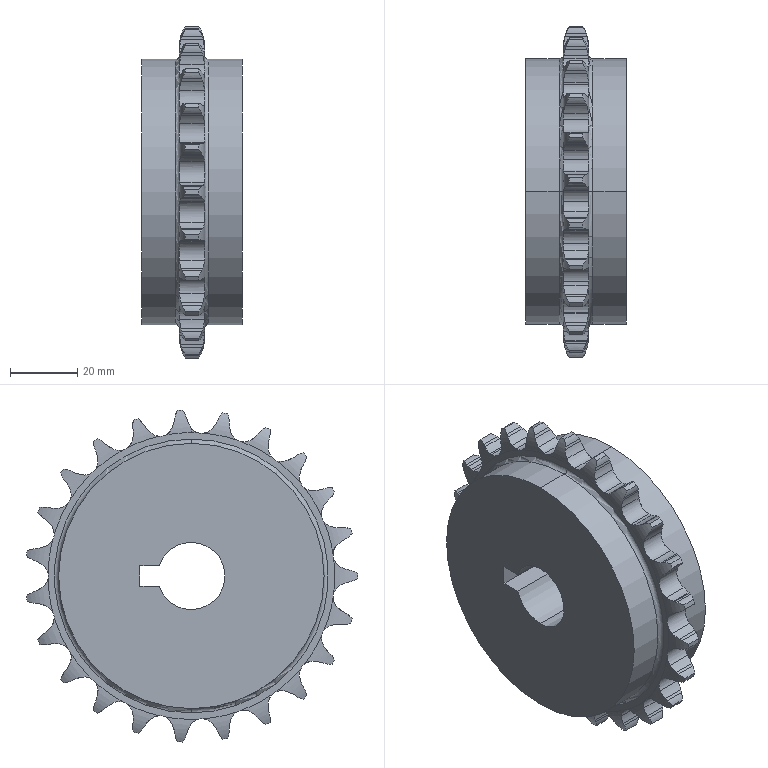Part | SolidWorks | features ICE 2, CirPattern 1, Cut 1, RefAxis 1, Revolution 1 | 1 solid | 262 faces | box 30 x 98.633 x 98.858 mm | volume 147727 mm3 | cylinder 157 | plane 53 | torus 52 | commonest cylinder face diameters 11.437 x49 20.732 x48 8.06 x30 99 x23 79 x4 20 x3